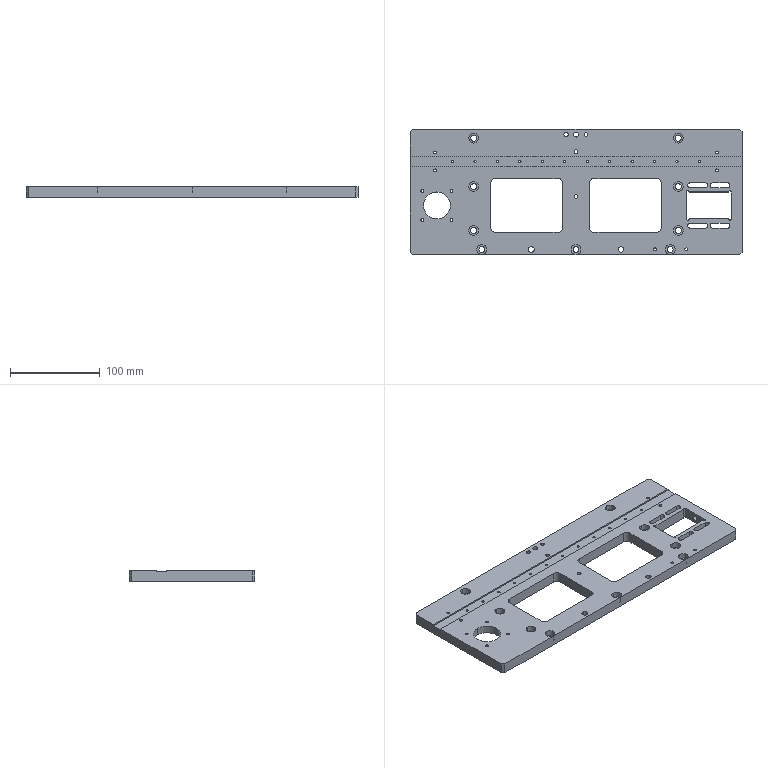Part | 1 solid | 179 faces | box 370 x 140 x 12 mm | volume 452920 mm3 | cylinder 126 | plane 53 | commonest cylinder face diameters 2.5 x24 3.3 x20 6.6 x18 11 x18 5.5 x12 10 x10